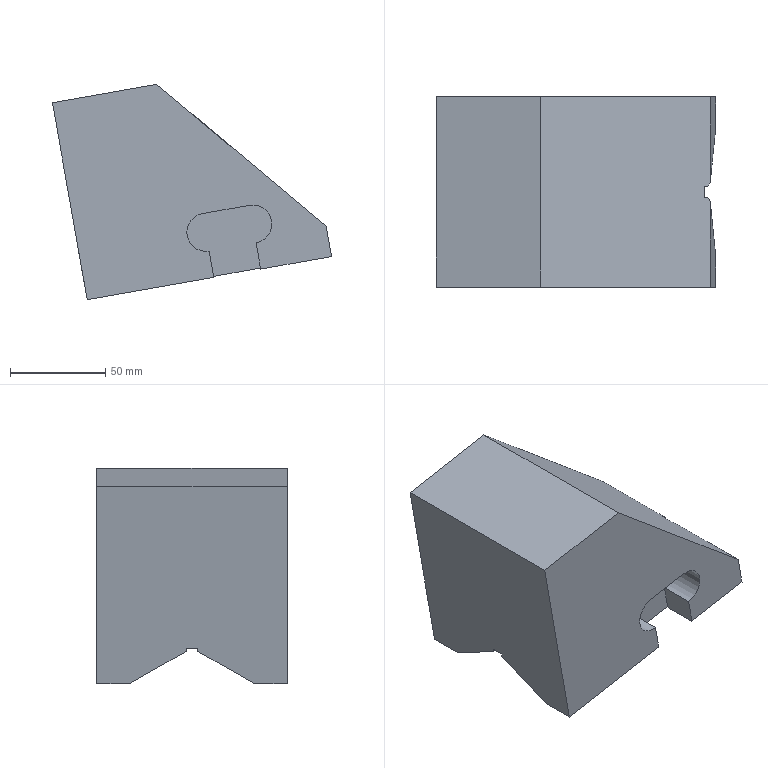Part | NX | features solid 2 | 1 solid | 28 faces | box 146.525 x 100 x 113.064 mm | volume 911913 mm3 | plane 24 | cylinder 4 | commonest cylinder face diameters 20 x4
STEP:
#1=CARTESIAN_POINT('',(885.872,-327.,12.071));
#2=VERTEX_POINT('',#1);
#3=CARTESIAN_POINT('',(885.872,-333.,12.071));
#4=VERTEX_POINT('',#3);
#5=CARTESIAN_POINT('',(885.872,-327.,12.071));
#6=DIRECTION('',(0.,-1.,0.));
#7=VECTOR('',#6,1000.);
#8=LINE('',#5,#7);
#9=EDGE_CURVE('',#2,#4,#8,.T.);
#10=ORIENTED_EDGE('',*,*,#9,.F.);
#11=CARTESIAN_POINT('',(887.604,-327.,10.618));
#12=VERTEX_POINT('',#11);
#13=CARTESIAN_POINT('',(888.817,-327.,9.6));
#14=DIRECTION('',(0.766,0.,-0.6428));
#15=VECTOR('',#14,1000.);
#16=LINE('',#13,#15);
#17=EDGE_CURVE('',#2,#12,#16,.T.);
#18=ORIENTED_EDGE('',*,*,#17,.T.);
#19=CARTESIAN_POINT('',(888.817,-324.899,9.6));
#20=VERTEX_POINT('',#19);
#21=CARTESIAN_POINT('',(901.667,-302.642,-1.182));
#22=DIRECTION('',(0.4611,0.7986,-0.3869));
#23=VECTOR('',#22,1000.);
#24=LINE('',#21,#23);
#25=EDGE_CURVE('',#12,#20,#24,.T.);
#26=ORIENTED_EDGE('',*,*,#25,.T.);
#27=CARTESIAN_POINT('',(888.817,-280.,9.6));
#28=VERTEX_POINT('',#27);
#29=CARTESIAN_POINT('',(888.817,-370.,9.6));
#30=DIRECTION('',(0.,-1.,0.));
#31=VECTOR('',#30,1000.);
#32=LINE('',#29,#31);
#33=EDGE_CURVE('',#28,#20,#32,.T.);
#34=ORIENTED_EDGE('',*,*,#33,.F.);
#35=CARTESIAN_POINT('',(799.874,-280.,84.232));
#36=VERTEX_POINT('',#35);
#37=CARTESIAN_POINT('',(835.289,-280.,54.515));
#38=DIRECTION('',(0.766,0.,-0.6428));
#39=VECTOR('',#38,1000.);
#40=LINE('',#37,#39);
#41=EDGE_CURVE('',#36,#28,#40,.T.);
#42=ORIENTED_EDGE('',*,*,#41,.F.);
#43=CARTESIAN_POINT('',(799.874,-380.,84.232));
#44=VERTEX_POINT('',#43);
#45=CARTESIAN_POINT('',(799.874,-290.,84.232));
#46=DIRECTION('',(0.,-1.,0.));
#47=VECTOR('',#46,1000.);
#48=LINE('',#45,#47);
#49=EDGE_CURVE('',#36,#44,#48,.T.);
#50=ORIENTED_EDGE('',*,*,#49,.T.);
#51=CARTESIAN_POINT('',(888.817,-380.,9.6));
#52=VERTEX_POINT('',#51);
#53=CARTESIAN_POINT('',(835.289,-380.,54.515));
#54=DIRECTION('',(-0.766,0.,0.6428));
#55=VECTOR('',#54,1000.);
#56=LINE('',#53,#55);
#57=EDGE_CURVE('',#52,#44,#56,.T.);
#58=ORIENTED_EDGE('',*,*,#57,.F.);
#59=CARTESIAN_POINT('',(888.817,-335.101,9.6));
#60=VERTEX_POINT('',#59);
#61=CARTESIAN_POINT('',(888.817,-370.,9.6));
#62=DIRECTION('',(0.,-1.,0.));
#63=VECTOR('',#62,1000.);
#64=LINE('',#61,#63);
#65=EDGE_CURVE('',#60,#52,#64,.T.);
#66=ORIENTED_EDGE('',*,*,#65,.F.);
#67=CARTESIAN_POINT('',(887.604,-333.,10.618));
#68=VERTEX_POINT('',#67);
#69=CARTESIAN_POINT('',(887.737,-333.23,10.507));
#70=DIRECTION('',(0.4611,-0.7986,-0.3869));
#71=VECTOR('',#70,1000.);
#72=LINE('',#69,#71);
#73=EDGE_CURVE('',#68,#60,#72,.T.);
#74=ORIENTED_EDGE('',*,*,#73,.F.);
#75=CARTESIAN_POINT('',(888.817,-333.,9.6));
#76=DIRECTION('',(-0.766,0.,0.6428));
#77=VECTOR('',#76,1000.);
#78=LINE('',#75,#77);
#79=EDGE_CURVE('',#68,#4,#78,.T.);
#80=ORIENTED_EDGE('',*,*,#79,.T.);
#81=EDGE_LOOP('',(#10,#18,#26,#34,#42,#50,#58,#66,#74,#80));
#82=FACE_BOUND('',#81,.T.);
#83=CARTESIAN_POINT('',(884.586,-333.,13.15));
#84=VERTEX_POINT('',#83);
#85=CARTESIAN_POINT('',(884.586,-327.,13.15));
#86=VERTEX_POINT('',#85);
#87=CARTESIAN_POINT('',(884.586,-290.,13.15));
#88=DIRECTION('',(0.,1.,0.));
#89=VECTOR('',#88,1000.);
#90=LINE('',#87,#89);
#91=EDGE_CURVE('',#84,#86,#90,.T.);
#92=ORIENTED_EDGE('',*,*,#91,.T.);
#93=ORIENTED_EDGE('',*,*,#91,.F.);
#94=EDGE_LOOP('',(#92,#93));
#95=FACE_BOUND('',#94,.T.);
#96=CARTESIAN_POINT('',(888.817,-290.,9.6));
#97=DIRECTION('',(0.6428,0.,0.766));
#98=DIRECTION('',(-0.766,0.,0.6428));
#99=AXIS2_PLACEMENT_3D('',#96,#97,#98);
#100=PLANE('',#99);
#101=ADVANCED_FACE('',(#82,#95),#100,.T.);
#102=CARTESIAN_POINT('',(885.033,-327.,10.165));
#103=VERTEX_POINT('',#102);
#104=CARTESIAN_POINT('',(760.314,-327.,-11.827));
#105=VERTEX_POINT('',#104);
#106=CARTESIAN_POINT('',(888.336,-327.,10.747));
#107=DIRECTION('',(-0.9848,0.,-0.1736));
#108=VECTOR('',#107,1000.);
#109=LINE('',#106,#108);
#110=EDGE_CURVE('',#103,#105,#109,.T.);
#111=ORIENTED_EDGE('',*,*,#110,.F.);
#112=CARTESIAN_POINT('',(888.336,-327.,10.747));
#113=DIRECTION('',(-0.9848,0.,-0.1736));
#114=VECTOR('',#113,1000.);
#115=LINE('',#112,#114);
#116=EDGE_CURVE('',#12,#103,#115,.T.);
#117=ORIENTED_EDGE('',*,*,#116,.F.);
#118=ORIENTED_EDGE('',*,*,#17,.F.);
#119=CARTESIAN_POINT('',(760.013,-327.,-10.121));
#120=VERTEX_POINT('',#119);
#121=CARTESIAN_POINT('',(888.036,-327.,12.453));
#122=DIRECTION('',(-0.9848,0.,-0.1736));
#123=VECTOR('',#122,1000.);
#124=LINE('',#121,#123);
#125=EDGE_CURVE('',#2,#120,#124,.T.);
#126=ORIENTED_EDGE('',*,*,#125,.T.);
#127=CARTESIAN_POINT('',(745.08,-327.,74.57));
#128=DIRECTION('',(0.1736,0.,-0.9848));
#129=VECTOR('',#128,1000.);
#130=LINE('',#127,#129);
#131=EDGE_CURVE('',#105,#120,#130,.F.);
#132=ORIENTED_EDGE('',*,*,#131,.F.);
#133=EDGE_LOOP('',(#111,#117,#118,#126,#132));
#134=FACE_BOUND('',#133,.T.);
#135=CARTESIAN_POINT('',(888.336,-327.,10.747));
#136=DIRECTION('',(0.,-1.,0.));
#137=DIRECTION('',(-0.1736,0.,0.9848));
#138=AXIS2_PLACEMENT_3D('',#135,#136,#137);
#139=PLANE('',#138);
#140=ADVANCED_FACE('',(#134),#139,.T.);
#141=ORIENTED_EDGE('',*,*,#125,.F.);
#142=ORIENTED_EDGE('',*,*,#9,.T.);
#143=CARTESIAN_POINT('',(760.013,-333.,-10.121));
#144=VERTEX_POINT('',#143);
#145=CARTESIAN_POINT('',(888.036,-333.,12.453));
#146=DIRECTION('',(-0.9848,0.,-0.1736));
#147=VECTOR('',#146,1000.);
#148=LINE('',#145,#147);
#149=EDGE_CURVE('',#4,#144,#148,.T.);
#150=ORIENTED_EDGE('',*,*,#149,.T.);
#151=CARTESIAN_POINT('',(760.013,-290.,-10.121));
#152=DIRECTION('',(0.,1.,0.));
#153=VECTOR('',#152,1000.);
#154=LINE('',#151,#153);
#155=EDGE_CURVE('',#120,#144,#154,.F.);
#156=ORIENTED_EDGE('',*,*,#155,.F.);
#157=EDGE_LOOP('',(#141,#142,#150,#156));
#158=FACE_BOUND('',#157,.T.);
#159=CARTESIAN_POINT('',(888.036,-327.,12.453));
#160=DIRECTION('',(0.1736,0.,-0.9848));
#161=DIRECTION('',(0.,-1.,0.));
#162=AXIS2_PLACEMENT_3D('',#159,#160,#161);
#163=PLANE('',#162);
#164=ADVANCED_FACE('',(#158),#163,.T.);
#165=ORIENTED_EDGE('',*,*,#149,.F.);
#166=ORIENTED_EDGE('',*,*,#79,.F.);
#167=CARTESIAN_POINT('',(760.314,-333.,-11.827));
#168=VERTEX_POINT('',#167);
#169=CARTESIAN_POINT('',(888.336,-333.,10.747));
#170=DIRECTION('',(-0.9848,0.,-0.1736));
#171=VECTOR('',#170,1000.);
#172=LINE('',#169,#171);
#173=EDGE_CURVE('',#68,#168,#172,.T.);
#174=ORIENTED_EDGE('',*,*,#173,.T.);
#175=CARTESIAN_POINT('',(745.08,-333.,74.57));
#176=DIRECTION('',(-0.1736,0.,0.9848));
#177=VECTOR('',#176,1000.);
#178=LINE('',#175,#177);
#179=EDGE_CURVE('',#144,#168,#178,.F.);
#180=ORIENTED_EDGE('',*,*,#179,.F.);
#181=EDGE_LOOP('',(#165,#166,#174,#180));
#182=FACE_BOUND('',#181,.T.);
#183=CARTESIAN_POINT('',(888.036,-333.,12.453));
#184=DIRECTION('',(0.,1.,0.));
#185=DIRECTION('',(0.1736,0.,-0.9848));
#186=AXIS2_PLACEMENT_3D('',#183,#184,#185);
#187=PLANE('',#186);
#188=ADVANCED_FACE('',(#182),#187,.T.);
#189=CARTESIAN_POINT('',(891.605,-380.,-6.211));
#190=VERTEX_POINT('',#189);
#191=CARTESIAN_POINT('',(882.488,-380.,45.491));
#192=DIRECTION('',(0.1736,0.,-0.9848));
#193=VECTOR('',#192,1000.);
#194=LINE('',#191,#193);
#195=EDGE_CURVE('',#52,#190,#194,.T.);
#196=ORIENTED_EDGE('',*,*,#195,.F.);
#197=ORIENTED_EDGE('',*,*,#57,.T.);
#198=CARTESIAN_POINT('',(745.08,-380.,74.57));
#199=VERTEX_POINT('',#198);
#200=CARTESIAN_POINT('',(809.09,-380.,85.857));
#201=DIRECTION('',(0.9848,0.,0.1736));
#202=VECTOR('',#201,1000.);
#203=LINE('',#200,#202);
#204=EDGE_CURVE('',#199,#44,#203,.T.);
#205=ORIENTED_EDGE('',*,*,#204,.F.);
#206=CARTESIAN_POINT('',(763.313,-380.,-28.832));
#207=VERTEX_POINT('',#206);
#208=CARTESIAN_POINT('',(745.08,-380.,74.57));
#209=DIRECTION('',(0.1736,0.,-0.9848));
#210=VECTOR('',#209,1000.);
#211=LINE('',#208,#210);
#212=EDGE_CURVE('',#207,#199,#211,.F.);
#213=ORIENTED_EDGE('',*,*,#212,.F.);
#214=CARTESIAN_POINT('',(829.784,-380.,-17.112));
#215=VERTEX_POINT('',#214);
#216=CARTESIAN_POINT('',(827.322,-380.,-17.546));
#217=DIRECTION('',(-0.9848,0.,-0.1736));
#218=VECTOR('',#217,1000.);
#219=LINE('',#216,#218);
#220=EDGE_CURVE('',#215,#207,#219,.T.);
#221=ORIENTED_EDGE('',*,*,#220,.F.);
#222=CARTESIAN_POINT('',(827.353,-380.,-3.324));
#223=VERTEX_POINT('',#222);
#224=CARTESIAN_POINT('',(820.668,-380.,34.591));
#225=DIRECTION('',(-0.1736,0.,0.9848));
#226=VECTOR('',#225,1000.);
#227=LINE('',#224,#226);
#228=EDGE_CURVE('',#215,#223,#227,.T.);
#229=ORIENTED_EDGE('',*,*,#228,.T.);
#230=CARTESIAN_POINT('',(823.88,-380.,16.372));
#231=VERTEX_POINT('',#230);
#232=CARTESIAN_POINT('',(825.617,-380.,6.524));
#233=DIRECTION('',(0.,-1.,0.));
#234=DIRECTION('',(0.,0.,-1.));
#235=AXIS2_PLACEMENT_3D('',#232,#233,#234);
#236=CIRCLE('',#235,10.);
#237=EDGE_CURVE('',#223,#231,#236,.F.);
#238=ORIENTED_EDGE('',*,*,#237,.T.);
#239=CARTESIAN_POINT('',(848.501,-380.,20.713));
#240=VERTEX_POINT('',#239);
#241=CARTESIAN_POINT('',(821.418,-380.,15.938));
#242=DIRECTION('',(0.9848,0.,0.1736));
#243=VECTOR('',#242,1000.);
#244=LINE('',#241,#243);
#245=EDGE_CURVE('',#231,#240,#244,.T.);
#246=ORIENTED_EDGE('',*,*,#245,.T.);
#247=CARTESIAN_POINT('',(851.974,-380.,1.017));
#248=VERTEX_POINT('',#247);
#249=CARTESIAN_POINT('',(850.237,-380.,10.865));
#250=DIRECTION('',(0.,-1.,0.));
#251=DIRECTION('',(0.,0.,-1.));
#252=AXIS2_PLACEMENT_3D('',#249,#250,#251);
#253=CIRCLE('',#252,10.);
#254=EDGE_CURVE('',#240,#248,#253,.F.);
#255=ORIENTED_EDGE('',*,*,#254,.T.);
#256=CARTESIAN_POINT('',(854.405,-380.,-12.77));
#257=VERTEX_POINT('',#256);
#258=CARTESIAN_POINT('',(845.288,-380.,38.932));
#259=DIRECTION('',(-0.1736,0.,0.9848));
#260=VECTOR('',#259,1000.);
#261=LINE('',#258,#260);
#262=EDGE_CURVE('',#257,#248,#261,.T.);
#263=ORIENTED_EDGE('',*,*,#262,.F.);
#264=CARTESIAN_POINT('',(827.322,-380.,-17.546));
#265=DIRECTION('',(-0.9848,0.,-0.1736));
#266=VECTOR('',#265,1000.);
#267=LINE('',#264,#266);
#268=EDGE_CURVE('',#190,#257,#267,.T.);
#269=ORIENTED_EDGE('',*,*,#268,.F.);
#270=EDGE_LOOP('',(#196,#197,#205,#213,#221,#229,#238,#246,#255,#263,#269));
#271=FACE_BOUND('',#270,.T.);
#272=CARTESIAN_POINT('',(818.206,-380.,34.157));
#273=DIRECTION('',(0.,-1.,0.));
#274=DIRECTION('',(0.9848,0.,0.1736));
#275=AXIS2_PLACEMENT_3D('',#272,#273,#274);
#276=PLANE('',#275);
#277=ADVANCED_FACE('',(#271),#276,.T.);
#278=CARTESIAN_POINT('',(829.784,-362.909,-17.112));
#279=VERTEX_POINT('',#278);
#280=CARTESIAN_POINT('',(763.313,-362.909,-28.832));
#281=VERTEX_POINT('',#280);
#282=CARTESIAN_POINT('',(891.335,-362.909,-6.259));
#283=DIRECTION('',(-0.9848,0.,-0.1736));
#284=VECTOR('',#283,1000.);
#285=LINE('',#282,#284);
#286=EDGE_CURVE('',#279,#281,#285,.T.);
#287=ORIENTED_EDGE('',*,*,#286,.F.);
#288=CARTESIAN_POINT('',(829.784,-370.,-17.112));
#289=DIRECTION('',(0.,-1.,0.));
#290=VECTOR('',#289,1000.);
#291=LINE('',#288,#290);
#292=EDGE_CURVE('',#279,#215,#291,.T.);
#293=ORIENTED_EDGE('',*,*,#292,.T.);
#294=ORIENTED_EDGE('',*,*,#220,.T.);
#295=CARTESIAN_POINT('',(763.313,-370.,-28.832));
#296=DIRECTION('',(0.,-1.,0.));
#297=VECTOR('',#296,1000.);
#298=LINE('',#295,#297);
#299=EDGE_CURVE('',#207,#281,#298,.F.);
#300=ORIENTED_EDGE('',*,*,#299,.T.);
#301=EDGE_LOOP('',(#287,#293,#294,#300));
#302=FACE_BOUND('',#301,.T.);
#303=CARTESIAN_POINT('',(827.322,-370.,-17.546));
#304=DIRECTION('',(0.1736,0.,-0.9848));
#305=DIRECTION('',(0.,-1.,0.));
#306=AXIS2_PLACEMENT_3D('',#303,#304,#305);
#307=PLANE('',#306);
#308=ADVANCED_FACE('',(#302),#307,.T.);
#309=ORIENTED_EDGE('',*,*,#173,.F.);
#310=ORIENTED_EDGE('',*,*,#73,.T.);
#311=CARTESIAN_POINT('',(891.605,-362.909,-6.211));
#312=VERTEX_POINT('',#311);
#313=CARTESIAN_POINT('',(888.606,-333.,10.795));
#314=DIRECTION('',(0.08682,-0.866,-0.4924));
#315=VECTOR('',#314,1000.);
#316=LINE('',#313,#315);
#317=EDGE_CURVE('',#60,#312,#316,.T.);
#318=ORIENTED_EDGE('',*,*,#317,.T.);
#319=CARTESIAN_POINT('',(854.405,-362.909,-12.77));
#320=VERTEX_POINT('',#319);
#321=CARTESIAN_POINT('',(891.335,-362.909,-6.259));
#322=DIRECTION('',(-0.9848,0.,-0.1736));
#323=VECTOR('',#322,1000.);
#324=LINE('',#321,#323);
#325=EDGE_CURVE('',#312,#320,#324,.T.);
#326=ORIENTED_EDGE('',*,*,#325,.T.);
#327=CARTESIAN_POINT('',(854.314,-362.,-12.254));
#328=VERTEX_POINT('',#327);
#329=CARTESIAN_POINT('',(851.406,-333.,4.235));
#330=DIRECTION('',(0.08682,-0.866,-0.4924));
#331=VECTOR('',#330,1000.);
#332=LINE('',#329,#331);
#333=EDGE_CURVE('',#328,#320,#332,.T.);
#334=ORIENTED_EDGE('',*,*,#333,.F.);
#335=CARTESIAN_POINT('',(829.693,-362.,-16.595));
#336=VERTEX_POINT('',#335);
#337=CARTESIAN_POINT('',(891.244,-362.,-5.742));
#338=DIRECTION('',(-0.9848,0.,-0.1736));
#339=VECTOR('',#338,1000.);
#340=LINE('',#337,#339);
#341=EDGE_CURVE('',#328,#336,#340,.T.);
#342=ORIENTED_EDGE('',*,*,#341,.T.);
#343=CARTESIAN_POINT('',(826.786,-333.,-0.1059));
#344=DIRECTION('',(0.08682,-0.866,-0.4924));
#345=VECTOR('',#344,1000.);
#346=LINE('',#343,#345);
#347=EDGE_CURVE('',#336,#279,#346,.T.);
#348=ORIENTED_EDGE('',*,*,#347,.T.);
#349=ORIENTED_EDGE('',*,*,#286,.T.);
#350=CARTESIAN_POINT('',(753.272,-262.762,28.109));
#351=DIRECTION('',(-0.08682,0.866,0.4924));
#352=VECTOR('',#351,1000.);
#353=LINE('',#350,#352);
#354=EDGE_CURVE('',#168,#281,#353,.F.);
#355=ORIENTED_EDGE('',*,*,#354,.F.);
#356=EDGE_LOOP('',(#309,#310,#318,#326,#334,#342,#348,#349,#355));
#357=FACE_BOUND('',#356,.T.);
#358=CARTESIAN_POINT('',(888.336,-333.,10.747));
#359=DIRECTION('',(0.1504,0.5,-0.8529));
#360=DIRECTION('',(0.08682,-0.866,-0.4924));
#361=AXIS2_PLACEMENT_3D('',#358,#359,#360);
#362=PLANE('',#361);
#363=ADVANCED_FACE('',(#357),#362,.T.);
#364=CARTESIAN_POINT('',(891.605,-297.091,-6.211));
#365=VERTEX_POINT('',#364);
#366=CARTESIAN_POINT('',(854.405,-297.091,-12.77));
#367=VERTEX_POINT('',#366);
#368=CARTESIAN_POINT('',(891.335,-297.091,-6.259));
#369=DIRECTION('',(-0.9848,0.,-0.1736));
#370=VECTOR('',#369,1000.);
#371=LINE('',#368,#370);
#372=EDGE_CURVE('',#365,#367,#371,.T.);
#373=ORIENTED_EDGE('',*,*,#372,.T.);
#374=CARTESIAN_POINT('',(854.405,-280.,-12.77));
#375=VERTEX_POINT('',#374);
#376=CARTESIAN_POINT('',(854.405,-370.,-12.77));
#377=DIRECTION('',(0.,1.,0.));
#378=VECTOR('',#377,1000.);
#379=LINE('',#376,#378);
#380=EDGE_CURVE('',#367,#375,#379,.T.);
#381=ORIENTED_EDGE('',*,*,#380,.T.);
#382=CARTESIAN_POINT('',(891.605,-280.,-6.211));
#383=VERTEX_POINT('',#382);
#384=CARTESIAN_POINT('',(827.322,-280.,-17.546));
#385=DIRECTION('',(0.9848,0.,0.1736));
#386=VECTOR('',#385,1000.);
#387=LINE('',#384,#386);
#388=EDGE_CURVE('',#375,#383,#387,.T.);
#389=ORIENTED_EDGE('',*,*,#388,.T.);
#390=CARTESIAN_POINT('',(891.605,-370.,-6.211));
#391=DIRECTION('',(0.,1.,0.));
#392=VECTOR('',#391,1000.);
#393=LINE('',#390,#392);
#394=EDGE_CURVE('',#365,#383,#393,.T.);
#395=ORIENTED_EDGE('',*,*,#394,.F.);
#396=EDGE_LOOP('',(#373,#381,#389,#395));
#397=FACE_BOUND('',#396,.T.);
#398=CARTESIAN_POINT('',(827.322,-370.,-17.546));
#399=DIRECTION('',(0.1736,0.,-0.9848));
#400=DIRECTION('',(0.,-1.,0.));
#401=AXIS2_PLACEMENT_3D('',#398,#399,#400);
#402=PLANE('',#401);
#403=ADVANCED_FACE('',(#397),#402,.T.);
#404=CARTESIAN_POINT('',(854.405,-370.,-12.77));
#405=DIRECTION('',(0.,-1.,0.));
#406=VECTOR('',#405,1000.);
#407=LINE('',#404,#406);
#408=EDGE_CURVE('',#320,#257,#407,.T.);
#409=ORIENTED_EDGE('',*,*,#408,.F.);
#410=ORIENTED_EDGE('',*,*,#325,.F.);
#411=CARTESIAN_POINT('',(891.605,-370.,-6.211));
#412=DIRECTION('',(0.,1.,0.));
#413=VECTOR('',#412,1000.);
#414=LINE('',#411,#413);
#415=EDGE_CURVE('',#190,#312,#414,.T.);
#416=ORIENTED_EDGE('',*,*,#415,.F.);
#417=ORIENTED_EDGE('',*,*,#268,.T.);
#418=EDGE_LOOP('',(#409,#410,#416,#417));
#419=FACE_BOUND('',#418,.T.);
#420=CARTESIAN_POINT('',(827.322,-370.,-17.546));
#421=DIRECTION('',(0.1736,0.,-0.9848));
#422=DIRECTION('',(0.,-1.,0.));
#423=AXIS2_PLACEMENT_3D('',#420,#421,#422);
#424=PLANE('',#423);
#425=ADVANCED_FACE('',(#419),#424,.T.);
#426=CARTESIAN_POINT('',(829.784,-297.091,-17.112));
#427=VERTEX_POINT('',#426);
#428=CARTESIAN_POINT('',(829.784,-280.,-17.112));
#429=VERTEX_POINT('',#428);
#430=CARTESIAN_POINT('',(829.784,-370.,-17.112));
#431=DIRECTION('',(0.,1.,0.));
#432=VECTOR('',#431,1000.);
#433=LINE('',#430,#432);
#434=EDGE_CURVE('',#427,#429,#433,.T.);
#435=ORIENTED_EDGE('',*,*,#434,.F.);
#436=CARTESIAN_POINT('',(763.313,-297.091,-28.832));
#437=VERTEX_POINT('',#436);
#438=CARTESIAN_POINT('',(891.335,-297.091,-6.259));
#439=DIRECTION('',(-0.9848,0.,-0.1736));
#440=VECTOR('',#439,1000.);
#441=LINE('',#438,#440);
#442=EDGE_CURVE('',#427,#437,#441,.T.);
#443=ORIENTED_EDGE('',*,*,#442,.T.);
#444=CARTESIAN_POINT('',(763.313,-280.,-28.832));
#445=VERTEX_POINT('',#444);
#446=CARTESIAN_POINT('',(763.313,-370.,-28.832));
#447=DIRECTION('',(0.,-1.,0.));
#448=VECTOR('',#447,1000.);
#449=LINE('',#446,#448);
#450=EDGE_CURVE('',#437,#445,#449,.F.);
#451=ORIENTED_EDGE('',*,*,#450,.T.);
#452=CARTESIAN_POINT('',(827.322,-280.,-17.546));
#453=DIRECTION('',(0.9848,0.,0.1736));
#454=VECTOR('',#453,1000.);
#455=LINE('',#452,#454);
#456=EDGE_CURVE('',#445,#429,#455,.T.);
#457=ORIENTED_EDGE('',*,*,#456,.T.);
#458=EDGE_LOOP('',(#435,#443,#451,#457));
#459=FACE_BOUND('',#458,.T.);
#460=CARTESIAN_POINT('',(827.322,-370.,-17.546));
#461=DIRECTION('',(0.1736,0.,-0.9848));
#462=DIRECTION('',(0.,-1.,0.));
#463=AXIS2_PLACEMENT_3D('',#460,#461,#462);
#464=PLANE('',#463);
#465=ADVANCED_FACE('',(#459),#464,.T.);
#466=ORIENTED_EDGE('',*,*,#415,.T.);
#467=ORIENTED_EDGE('',*,*,#317,.F.);
#468=ORIENTED_EDGE('',*,*,#65,.T.);
#469=ORIENTED_EDGE('',*,*,#195,.T.);
#470=EDGE_LOOP('',(#466,#467,#468,#469));
#471=FACE_BOUND('',#470,.T.);
#472=CARTESIAN_POINT('',(882.488,-370.,45.491));
#473=DIRECTION('',(0.9848,0.,0.1736));
#474=DIRECTION('',(0.,1.,0.));
#475=AXIS2_PLACEMENT_3D('',#472,#473,#474);
#476=PLANE('',#475);
#477=ADVANCED_FACE('',(#471),#476,.T.);
#478=ORIENTED_EDGE('',*,*,#33,.T.);
#479=CARTESIAN_POINT('',(891.605,-297.091,-6.211));
#480=DIRECTION('',(-0.08682,-0.866,0.4924));
#481=VECTOR('',#480,1000.);
#482=LINE('',#479,#481);
#483=EDGE_CURVE('',#365,#20,#482,.T.);
#484=ORIENTED_EDGE('',*,*,#483,.F.);
#485=ORIENTED_EDGE('',*,*,#394,.T.);
#486=CARTESIAN_POINT('',(882.488,-280.,45.491));
#487=DIRECTION('',(-0.1736,0.,0.9848));
#488=VECTOR('',#487,1000.);
#489=LINE('',#486,#488);
#490=EDGE_CURVE('',#383,#28,#489,.T.);
#491=ORIENTED_EDGE('',*,*,#490,.T.);
#492=EDGE_LOOP('',(#478,#484,#485,#491));
#493=FACE_BOUND('',#492,.T.);
#494=CARTESIAN_POINT('',(882.488,-370.,45.491));
#495=DIRECTION('',(0.9848,0.,0.1736));
#496=DIRECTION('',(0.,1.,0.));
#497=AXIS2_PLACEMENT_3D('',#494,#495,#496);
#498=PLANE('',#497);
#499=ADVANCED_FACE('',(#493),#498,.T.);
#500=ORIENTED_EDGE('',*,*,#212,.T.);
#501=CARTESIAN_POINT('',(745.08,-280.,74.57));
#502=VERTEX_POINT('',#501);
#503=CARTESIAN_POINT('',(745.08,-290.,74.57));
#504=DIRECTION('',(0.,1.,0.));
#505=VECTOR('',#504,1000.);
#506=LINE('',#503,#505);
#507=EDGE_CURVE('',#502,#199,#506,.F.);
#508=ORIENTED_EDGE('',*,*,#507,.F.);
#509=CARTESIAN_POINT('',(745.08,-280.,74.57));
#510=DIRECTION('',(-0.1736,0.,0.9848));
#511=VECTOR('',#510,1000.);
#512=LINE('',#509,#511);
#513=EDGE_CURVE('',#502,#445,#512,.F.);
#514=ORIENTED_EDGE('',*,*,#513,.T.);
#515=ORIENTED_EDGE('',*,*,#450,.F.);
#516=CARTESIAN_POINT('',(759.288,-337.238,-6.006));
#517=DIRECTION('',(0.08682,0.866,-0.4924));
#518=VECTOR('',#517,1000.);
#519=LINE('',#516,#518);
#520=EDGE_CURVE('',#437,#105,#519,.F.);
#521=ORIENTED_EDGE('',*,*,#520,.T.);
#522=ORIENTED_EDGE('',*,*,#131,.T.);
#523=ORIENTED_EDGE('',*,*,#155,.T.);
#524=ORIENTED_EDGE('',*,*,#179,.T.);
#525=ORIENTED_EDGE('',*,*,#354,.T.);
#526=ORIENTED_EDGE('',*,*,#299,.F.);
#527=EDGE_LOOP('',(#500,#508,#514,#515,#521,#522,#523,#524,#525,#526));
#528=FACE_BOUND('',#527,.T.);
#529=CARTESIAN_POINT('',(745.08,-290.,74.57));
#530=DIRECTION('',(0.9848,0.,0.1736));
#531=DIRECTION('',(0.,-1.,0.));
#532=AXIS2_PLACEMENT_3D('',#529,#530,#531);
#533=PLANE('',#532);
#534=ADVANCED_FACE('',(#528),#533,.F.);
#535=ORIENTED_EDGE('',*,*,#41,.T.);
#536=ORIENTED_EDGE('',*,*,#490,.F.);
#537=ORIENTED_EDGE('',*,*,#388,.F.);
#538=CARTESIAN_POINT('',(851.974,-280.,1.017));
#539=VERTEX_POINT('',#538);
#540=CARTESIAN_POINT('',(845.288,-280.,38.932));
#541=DIRECTION('',(-0.1736,0.,0.9848));
#542=VECTOR('',#541,1000.);
#543=LINE('',#540,#542);
#544=EDGE_CURVE('',#375,#539,#543,.T.);
#545=ORIENTED_EDGE('',*,*,#544,.T.);
#546=CARTESIAN_POINT('',(848.501,-280.,20.713));
#547=VERTEX_POINT('',#546);
#548=CARTESIAN_POINT('',(850.237,-280.,10.865));
#549=DIRECTION('',(0.,1.,0.));
#550=DIRECTION('',(0.,0.,1.));
#551=AXIS2_PLACEMENT_3D('',#548,#549,#550);
#552=CIRCLE('',#551,10.);
#553=EDGE_CURVE('',#547,#539,#552,.T.);
#554=ORIENTED_EDGE('',*,*,#553,.F.);
#555=CARTESIAN_POINT('',(823.88,-280.,16.372));
#556=VERTEX_POINT('',#555);
#557=CARTESIAN_POINT('',(821.418,-280.,15.938));
#558=DIRECTION('',(-0.9848,0.,-0.1736));
#559=VECTOR('',#558,1000.);
#560=LINE('',#557,#559);
#561=EDGE_CURVE('',#547,#556,#560,.T.);
#562=ORIENTED_EDGE('',*,*,#561,.T.);
#563=CARTESIAN_POINT('',(827.353,-280.,-3.324));
#564=VERTEX_POINT('',#563);
#565=CARTESIAN_POINT('',(825.617,-280.,6.524));
#566=DIRECTION('',(0.,1.,0.));
#567=DIRECTION('',(0.,0.,1.));
#568=AXIS2_PLACEMENT_3D('',#565,#566,#567);
#569=CIRCLE('',#568,10.);
#570=EDGE_CURVE('',#564,#556,#569,.T.);
#571=ORIENTED_EDGE('',*,*,#570,.F.);
#572=CARTESIAN_POINT('',(820.668,-280.,34.591));
#573=DIRECTION('',(-0.1736,0.,0.9848));
#574=VECTOR('',#573,1000.);
#575=LINE('',#572,#574);
#576=EDGE_CURVE('',#429,#564,#575,.T.);
#577=ORIENTED_EDGE('',*,*,#576,.F.);
#578=ORIENTED_EDGE('',*,*,#456,.F.);
#579=ORIENTED_EDGE('',*,*,#513,.F.);
#580=CARTESIAN_POINT('',(745.08,-280.,74.57));
#581=DIRECTION('',(0.9848,0.,0.1736));
#582=VECTOR('',#581,1000.);
#583=LINE('',#580,#582);
#584=EDGE_CURVE('',#502,#36,#583,.T.);
#585=ORIENTED_EDGE('',*,*,#584,.T.);
#586=EDGE_LOOP('',(#535,#536,#537,#545,#554,#562,#571,#577,#578,#579,#585));
#587=FACE_BOUND('',#586,.T.);
#588=CARTESIAN_POINT('',(818.206,-280.,34.157));
#589=DIRECTION('',(0.,1.,0.));
#590=DIRECTION('',(-0.9848,0.,-0.1736));
#591=AXIS2_PLACEMENT_3D('',#588,#589,#590);
#592=PLANE('',#591);
#593=ADVANCED_FACE('',(#587),#592,.T.);
#594=ORIENTED_EDGE('',*,*,#483,.T.);
#595=ORIENTED_EDGE('',*,*,#25,.F.);
#596=ORIENTED_EDGE('',*,*,#116,.T.);
#597=CARTESIAN_POINT('',(887.531,-322.672,8.068));
#598=VERTEX_POINT('',#597);
#599=CARTESIAN_POINT('',(900.315,-300.531,-2.658));
#600=DIRECTION('',(-0.4611,-0.7986,0.3869));
#601=VECTOR('',#600,1000.);
#602=LINE('',#599,#601);
#603=EDGE_CURVE('',#598,#103,#602,.T.);
#604=ORIENTED_EDGE('',*,*,#603,.F.);
#605=ORIENTED_EDGE('',*,*,#603,.T.);
#606=ORIENTED_EDGE('',*,*,#110,.T.);
#607=ORIENTED_EDGE('',*,*,#520,.F.);
#608=ORIENTED_EDGE('',*,*,#442,.F.);
#609=CARTESIAN_POINT('',(829.693,-298.,-16.595));
#610=VERTEX_POINT('',#609);
#611=CARTESIAN_POINT('',(829.784,-297.091,-17.112));
#612=DIRECTION('',(0.08682,0.866,-0.4924));
#613=VECTOR('',#612,1000.);
#614=LINE('',#611,#613);
#615=EDGE_CURVE('',#610,#427,#614,.T.);
#616=ORIENTED_EDGE('',*,*,#615,.F.);
#617=CARTESIAN_POINT('',(854.314,-298.,-12.254));
#618=VERTEX_POINT('',#617);
#619=CARTESIAN_POINT('',(891.244,-298.,-5.742));
#620=DIRECTION('',(0.9848,0.,0.1736));
#621=VECTOR('',#620,1000.);
#622=LINE('',#619,#621);
#623=EDGE_CURVE('',#610,#618,#622,.T.);
#624=ORIENTED_EDGE('',*,*,#623,.T.);
#625=CARTESIAN_POINT('',(854.405,-297.091,-12.77));
#626=DIRECTION('',(0.08682,0.866,-0.4924));
#627=VECTOR('',#626,1000.);
#628=LINE('',#625,#627);
#629=EDGE_CURVE('',#618,#367,#628,.T.);
#630=ORIENTED_EDGE('',*,*,#629,.T.);
#631=ORIENTED_EDGE('',*,*,#372,.F.);
#632=EDGE_LOOP('',(#594,#595,#596,#604,#605,#606,#607,#608,#616,#624,#630,#631));
#633=FACE_BOUND('',#632,.T.);
#634=CARTESIAN_POINT('',(891.335,-297.091,-6.259));
#635=DIRECTION('',(0.1504,-0.5,-0.8529));
#636=DIRECTION('',(-0.08682,-0.866,0.4924));
#637=AXIS2_PLACEMENT_3D('',#634,#635,#636);
#638=PLANE('',#637);
#639=ADVANCED_FACE('',(#633),#638,.T.);
#640=ORIENTED_EDGE('',*,*,#570,.T.);
#641=CARTESIAN_POINT('',(823.88,-298.,16.372));
#642=VERTEX_POINT('',#641);
#643=CARTESIAN_POINT('',(823.88,-298.,16.372));
#644=DIRECTION('',(0.,1.,0.));
#645=VECTOR('',#644,1000.);
#646=LINE('',#643,#645);
#647=EDGE_CURVE('',#642,#556,#646,.T.);
#648=ORIENTED_EDGE('',*,*,#647,.F.);
#649=CARTESIAN_POINT('',(827.353,-298.,-3.324));
#650=VERTEX_POINT('',#649);
#651=CARTESIAN_POINT('',(825.617,-298.,6.524));
#652=DIRECTION('',(0.,1.,0.));
#653=DIRECTION('',(-0.9659,0.,0.2588));
#654=AXIS2_PLACEMENT_3D('',#651,#652,#653);
#655=CIRCLE('',#654,10.);
#656=EDGE_CURVE('',#650,#642,#655,.T.);
#657=ORIENTED_EDGE('',*,*,#656,.F.);
#658=CARTESIAN_POINT('',(827.353,-298.,-3.324));
#659=DIRECTION('',(0.,1.,0.));
#660=VECTOR('',#659,1000.);
#661=LINE('',#658,#660);
#662=EDGE_CURVE('',#650,#564,#661,.T.);
#663=ORIENTED_EDGE('',*,*,#662,.T.);
#664=EDGE_LOOP('',(#640,#648,#657,#663));
#665=FACE_BOUND('',#664,.T.);
#666=CARTESIAN_POINT('',(825.617,-298.,6.524));
#667=DIRECTION('',(0.,1.,0.));
#668=DIRECTION('',(-0.9397,0.,0.342));
#669=AXIS2_PLACEMENT_3D('',#666,#667,#668);
#670=CYLINDRICAL_SURFACE('',#669,10.);
#671=ADVANCED_FACE('',(#665),#670,.F.);
#672=ORIENTED_EDGE('',*,*,#561,.F.);
#673=CARTESIAN_POINT('',(848.501,-298.,20.713));
#674=VERTEX_POINT('',#673);
#675=CARTESIAN_POINT('',(848.501,-298.,20.713));
#676=DIRECTION('',(0.,1.,0.));
#677=VECTOR('',#676,1000.);
#678=LINE('',#675,#677);
#679=EDGE_CURVE('',#674,#547,#678,.T.);
#680=ORIENTED_EDGE('',*,*,#679,.F.);
#681=CARTESIAN_POINT('',(848.501,-298.,20.713));
#682=DIRECTION('',(-0.9848,0.,-0.1736));
#683=VECTOR('',#682,1000.);
#684=LINE('',#681,#683);
#685=EDGE_CURVE('',#674,#642,#684,.T.);
#686=ORIENTED_EDGE('',*,*,#685,.T.);
#687=ORIENTED_EDGE('',*,*,#647,.T.);
#688=EDGE_LOOP('',(#672,#680,#686,#687));
#689=FACE_BOUND('',#688,.T.);
#690=CARTESIAN_POINT('',(848.501,-298.,20.713));
#691=DIRECTION('',(0.1736,0.,-0.9848));
#692=DIRECTION('',(-0.9848,0.,-0.1736));
#693=AXIS2_PLACEMENT_3D('',#690,#691,#692);
#694=PLANE('',#693);
#695=ADVANCED_FACE('',(#689),#694,.T.);
#696=ORIENTED_EDGE('',*,*,#553,.T.);
#697=CARTESIAN_POINT('',(851.974,-298.,1.017));
#698=VERTEX_POINT('',#697);
#699=CARTESIAN_POINT('',(851.974,-298.,1.017));
#700=DIRECTION('',(0.,1.,0.));
#701=VECTOR('',#700,1000.);
#702=LINE('',#699,#701);
#703=EDGE_CURVE('',#698,#539,#702,.T.);
#704=ORIENTED_EDGE('',*,*,#703,.F.);
#705=CARTESIAN_POINT('',(850.237,-298.,10.865));
#706=DIRECTION('',(0.,1.,0.));
#707=DIRECTION('',(-0.9659,0.,0.2588));
#708=AXIS2_PLACEMENT_3D('',#705,#706,#707);
#709=CIRCLE('',#708,10.);
#710=EDGE_CURVE('',#674,#698,#709,.T.);
#711=ORIENTED_EDGE('',*,*,#710,.F.);
#712=ORIENTED_EDGE('',*,*,#679,.T.);
#713=EDGE_LOOP('',(#696,#704,#711,#712));
#714=FACE_BOUND('',#713,.T.);
#715=CARTESIAN_POINT('',(850.237,-298.,10.865));
#716=DIRECTION('',(0.,1.,0.));
#717=DIRECTION('',(-0.9397,0.,0.342));
#718=AXIS2_PLACEMENT_3D('',#715,#716,#717);
#719=CYLINDRICAL_SURFACE('',#718,10.);
#720=ADVANCED_FACE('',(#714),#719,.F.);
#721=ORIENTED_EDGE('',*,*,#710,.T.);
#722=CARTESIAN_POINT('',(857.183,-298.,-28.527));
#723=DIRECTION('',(-0.1736,0.,0.9848));
#724=VECTOR('',#723,1000.);
#725=LINE('',#722,#724);
#726=EDGE_CURVE('',#618,#698,#725,.T.);
#727=ORIENTED_EDGE('',*,*,#726,.F.);
#728=ORIENTED_EDGE('',*,*,#623,.F.);
#729=CARTESIAN_POINT('',(832.563,-298.,-32.868));
#730=DIRECTION('',(-0.1736,0.,0.9848));
#731=VECTOR('',#730,1000.);
#732=LINE('',#729,#731);
#733=EDGE_CURVE('',#610,#650,#732,.T.);
#734=ORIENTED_EDGE('',*,*,#733,.T.);
#735=ORIENTED_EDGE('',*,*,#656,.T.);
#736=ORIENTED_EDGE('',*,*,#685,.F.);
#737=EDGE_LOOP('',(#721,#727,#728,#734,#735,#736));
#738=FACE_BOUND('',#737,.T.);
#739=CARTESIAN_POINT('',(825.617,-298.,6.524));
#740=DIRECTION('',(0.,1.,0.));
#741=DIRECTION('',(-0.9397,0.,0.342));
#742=AXIS2_PLACEMENT_3D('',#739,#740,#741);
#743=PLANE('',#742);
#744=ADVANCED_FACE('',(#738),#743,.T.);
#745=ORIENTED_EDGE('',*,*,#434,.T.);
#746=ORIENTED_EDGE('',*,*,#576,.T.);
#747=ORIENTED_EDGE('',*,*,#662,.F.);
#748=ORIENTED_EDGE('',*,*,#733,.F.);
#749=ORIENTED_EDGE('',*,*,#615,.T.);
#750=EDGE_LOOP('',(#745,#746,#747,#748,#749));
#751=FACE_BOUND('',#750,.T.);
#752=CARTESIAN_POINT('',(832.563,-298.,-32.868));
#753=DIRECTION('',(-0.9848,0.,-0.1736));
#754=DIRECTION('',(-0.1736,0.,0.9848));
#755=AXIS2_PLACEMENT_3D('',#752,#753,#754);
#756=PLANE('',#755);
#757=ADVANCED_FACE('',(#751),#756,.F.);
#758=ORIENTED_EDGE('',*,*,#629,.F.);
#759=ORIENTED_EDGE('',*,*,#726,.T.);
#760=ORIENTED_EDGE('',*,*,#703,.T.);
#761=ORIENTED_EDGE('',*,*,#544,.F.);
#762=ORIENTED_EDGE('',*,*,#380,.F.);
#763=EDGE_LOOP('',(#758,#759,#760,#761,#762));
#764=FACE_BOUND('',#763,.T.);
#765=CARTESIAN_POINT('',(857.183,-298.,-28.527));
#766=DIRECTION('',(-0.9848,0.,-0.1736));
#767=DIRECTION('',(-0.1736,0.,0.9848));
#768=AXIS2_PLACEMENT_3D('',#765,#766,#767);
#769=PLANE('',#768);
#770=ADVANCED_FACE('',(#764),#769,.T.);
#771=ORIENTED_EDGE('',*,*,#245,.F.);
#772=CARTESIAN_POINT('',(823.88,-362.,16.372));
#773=VERTEX_POINT('',#772);
#774=CARTESIAN_POINT('',(823.88,-362.,16.372));
#775=DIRECTION('',(0.,-1.,0.));
#776=VECTOR('',#775,1000.);
#777=LINE('',#774,#776);
#778=EDGE_CURVE('',#773,#231,#777,.T.);
#779=ORIENTED_EDGE('',*,*,#778,.F.);
#780=CARTESIAN_POINT('',(848.501,-362.,20.713));
#781=VERTEX_POINT('',#780);
#782=CARTESIAN_POINT('',(823.88,-362.,16.372));
#783=DIRECTION('',(0.9848,0.,0.1736));
#784=VECTOR('',#783,1000.);
#785=LINE('',#782,#784);
#786=EDGE_CURVE('',#773,#781,#785,.T.);
#787=ORIENTED_EDGE('',*,*,#786,.T.);
#788=CARTESIAN_POINT('',(848.501,-370.,20.713));
#789=DIRECTION('',(0.,1.,0.));
#790=VECTOR('',#789,1000.);
#791=LINE('',#788,#790);
#792=EDGE_CURVE('',#240,#781,#791,.T.);
#793=ORIENTED_EDGE('',*,*,#792,.F.);
#794=EDGE_LOOP('',(#771,#779,#787,#793));
#795=FACE_BOUND('',#794,.T.);
#796=CARTESIAN_POINT('',(823.88,-362.,16.372));
#797=DIRECTION('',(0.1736,0.,-0.9848));
#798=DIRECTION('',(-0.9848,0.,-0.1736));
#799=AXIS2_PLACEMENT_3D('',#796,#797,#798);
#800=PLANE('',#799);
#801=ADVANCED_FACE('',(#795),#800,.T.);
#802=CARTESIAN_POINT('',(827.353,-362.,-3.324));
#803=VERTEX_POINT('',#802);
#804=CARTESIAN_POINT('',(827.353,-370.,-3.324));
#805=DIRECTION('',(0.,1.,0.));
#806=VECTOR('',#805,1000.);
#807=LINE('',#804,#806);
#808=EDGE_CURVE('',#223,#803,#807,.T.);
#809=ORIENTED_EDGE('',*,*,#808,.F.);
#810=ORIENTED_EDGE('',*,*,#228,.F.);
#811=ORIENTED_EDGE('',*,*,#292,.F.);
#812=ORIENTED_EDGE('',*,*,#347,.F.);
#813=CARTESIAN_POINT('',(832.563,-362.,-32.868));
#814=DIRECTION('',(-0.1736,0.,0.9848));
#815=VECTOR('',#814,1000.);
#816=LINE('',#813,#815);
#817=EDGE_CURVE('',#336,#803,#816,.T.);
#818=ORIENTED_EDGE('',*,*,#817,.T.);
#819=EDGE_LOOP('',(#809,#810,#811,#812,#818));
#820=FACE_BOUND('',#819,.T.);
#821=CARTESIAN_POINT('',(832.563,-362.,-32.868));
#822=DIRECTION('',(0.9848,0.,0.1736));
#823=DIRECTION('',(0.1736,0.,-0.9848));
#824=AXIS2_PLACEMENT_3D('',#821,#822,#823);
#825=PLANE('',#824);
#826=ADVANCED_FACE('',(#820),#825,.T.);
#827=ORIENTED_EDGE('',*,*,#262,.T.);
#828=CARTESIAN_POINT('',(851.974,-362.,1.017));
#829=VERTEX_POINT('',#828);
#830=CARTESIAN_POINT('',(851.974,-370.,1.017));
#831=DIRECTION('',(0.,1.,0.));
#832=VECTOR('',#831,1000.);
#833=LINE('',#830,#832);
#834=EDGE_CURVE('',#248,#829,#833,.T.);
#835=ORIENTED_EDGE('',*,*,#834,.T.);
#836=CARTESIAN_POINT('',(851.974,-362.,1.017));
#837=DIRECTION('',(-0.1736,0.,0.9848));
#838=VECTOR('',#837,1000.);
#839=LINE('',#836,#838);
#840=EDGE_CURVE('',#328,#829,#839,.T.);
#841=ORIENTED_EDGE('',*,*,#840,.F.);
#842=ORIENTED_EDGE('',*,*,#333,.T.);
#843=ORIENTED_EDGE('',*,*,#408,.T.);
#844=EDGE_LOOP('',(#827,#835,#841,#842,#843));
#845=FACE_BOUND('',#844,.T.);
#846=CARTESIAN_POINT('',(851.974,-362.,1.017));
#847=DIRECTION('',(0.9848,0.,0.1736));
#848=DIRECTION('',(0.1736,0.,-0.9848));
#849=AXIS2_PLACEMENT_3D('',#846,#847,#848);
#850=PLANE('',#849);
#851=ADVANCED_FACE('',(#845),#850,.F.);
#852=CARTESIAN_POINT('',(850.237,-362.,10.865));
#853=DIRECTION('',(0.,1.,0.));
#854=DIRECTION('',(-0.9659,0.,0.2588));
#855=AXIS2_PLACEMENT_3D('',#852,#853,#854);
#856=CIRCLE('',#855,10.);
#857=EDGE_CURVE('',#781,#829,#856,.T.);
#858=ORIENTED_EDGE('',*,*,#857,.F.);
#859=ORIENTED_EDGE('',*,*,#786,.F.);
#860=CARTESIAN_POINT('',(825.617,-362.,6.524));
#861=DIRECTION('',(0.,1.,0.));
#862=DIRECTION('',(-0.9659,0.,0.2588));
#863=AXIS2_PLACEMENT_3D('',#860,#861,#862);
#864=CIRCLE('',#863,10.);
#865=EDGE_CURVE('',#803,#773,#864,.T.);
#866=ORIENTED_EDGE('',*,*,#865,.F.);
#867=ORIENTED_EDGE('',*,*,#817,.F.);
#868=ORIENTED_EDGE('',*,*,#341,.F.);
#869=ORIENTED_EDGE('',*,*,#840,.T.);
#870=EDGE_LOOP('',(#858,#859,#866,#867,#868,#869));
#871=FACE_BOUND('',#870,.T.);
#872=CARTESIAN_POINT('',(820.407,-362.,36.068));
#873=DIRECTION('',(0.,-1.,0.));
#874=DIRECTION('',(-0.9397,0.,0.342));
#875=AXIS2_PLACEMENT_3D('',#872,#873,#874);
#876=PLANE('',#875);
#877=ADVANCED_FACE('',(#871),#876,.T.);
#878=ORIENTED_EDGE('',*,*,#857,.T.);
#879=ORIENTED_EDGE('',*,*,#834,.F.);
#880=ORIENTED_EDGE('',*,*,#254,.F.);
#881=ORIENTED_EDGE('',*,*,#792,.T.);
#882=EDGE_LOOP('',(#878,#879,#880,#881));
#883=FACE_BOUND('',#882,.T.);
#884=CARTESIAN_POINT('',(850.237,-370.,10.865));
#885=DIRECTION('',(0.,1.,0.));
#886=DIRECTION('',(-0.9397,0.,0.342));
#887=AXIS2_PLACEMENT_3D('',#884,#885,#886);
#888=CYLINDRICAL_SURFACE('',#887,10.);
#889=ADVANCED_FACE('',(#883),#888,.F.);
#890=ORIENTED_EDGE('',*,*,#865,.T.);
#891=ORIENTED_EDGE('',*,*,#778,.T.);
#892=ORIENTED_EDGE('',*,*,#237,.F.);
#893=ORIENTED_EDGE('',*,*,#808,.T.);
#894=EDGE_LOOP('',(#890,#891,#892,#893));
#895=FACE_BOUND('',#894,.T.);
#896=CARTESIAN_POINT('',(825.617,-370.,6.524));
#897=DIRECTION('',(0.,1.,0.));
#898=DIRECTION('',(-0.9397,0.,0.342));
#899=AXIS2_PLACEMENT_3D('',#896,#897,#898);
#900=CYLINDRICAL_SURFACE('',#899,10.);
#901=ADVANCED_FACE('',(#895),#900,.F.);
#902=ORIENTED_EDGE('',*,*,#49,.F.);
#903=ORIENTED_EDGE('',*,*,#584,.F.);
#904=ORIENTED_EDGE('',*,*,#507,.T.);
#905=ORIENTED_EDGE('',*,*,#204,.T.);
#906=EDGE_LOOP('',(#902,#903,#904,#905));
#907=FACE_BOUND('',#906,.T.);
#908=CARTESIAN_POINT('',(745.08,-290.,74.57));
#909=DIRECTION('',(0.1736,0.,-0.9848));
#910=DIRECTION('',(0.9848,0.,0.1736));
#911=AXIS2_PLACEMENT_3D('',#908,#909,#910);
#912=PLANE('',#911);
#913=ADVANCED_FACE('',(#907),#912,.F.);
#914=CLOSED_SHELL('',(#101,#140,#164,#188,#277,#308,#363,#403,#425,#465,#477,#499,#534,#593,#639,#671,#695,#720,#744,#757,#770,#801,#826,#851,#877,#889,#901,#913));
#915=MANIFOLD_SOLID_BREP('',#914);
#916=(LENGTH_UNIT()NAMED_UNIT(*)SI_UNIT(.MILLI.,.METRE.));
#917=UNCERTAINTY_MEASURE_WITH_UNIT(LENGTH_MEASURE(0.00001),#916,'','');
#918=(NAMED_UNIT(*)PLANE_ANGLE_UNIT()SI_UNIT($,.RADIAN.));
#919=(NAMED_UNIT(*)SI_UNIT($,.STERADIAN.)SOLID_ANGLE_UNIT());
#920=(GEOMETRIC_REPRESENTATION_CONTEXT(3)GLOBAL_UNCERTAINTY_ASSIGNED_CONTEXT((#917))GLOBAL_UNIT_ASSIGNED_CONTEXT((#916,#918,#919))REPRESENTATION_CONTEXT('',''));
#921=ADVANCED_BREP_SHAPE_REPRESENTATION('',(#915),#920);